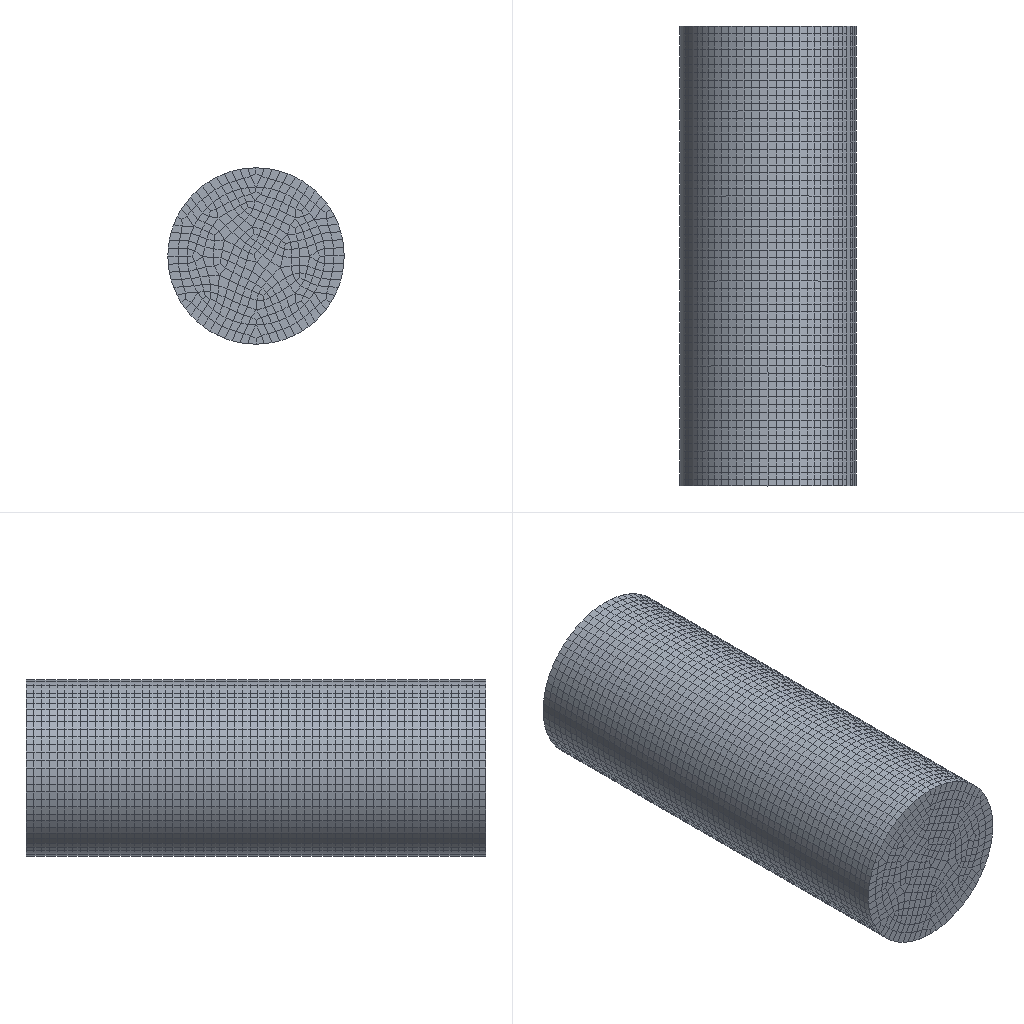Simulation study | ansys workbench
Set-up summary:
category,name,step,type,value,unit,region
solver,ansys_workbench
units,SI m-kg-s (Pa),,stated,"/units,MKS"
analysis,deck-1/LS1,,steady-state thermal
load_step,deck-1/LS1,deck-1/LS1,steady-state thermal,nsubst=1; time=1
analysis,deck-2/LS1,,transient thermal
load_step,deck-2/LS1,deck-2/LS1,transient thermal,nsubst=100; time=10
analysis,deck-3/LS1,,transient thermal
load_step,deck-3/LS1,deck-3/LS1,transient thermal,nsubst=100; time=100
mesh,deck-1.dat,,nodes,46128
mesh,deck-1.dat,,elements,12591
element_type,SOLID90,,,8511,,deck-1.dat
element_type,SURF152,,,4080,,deck-1.dat
mesh,deck-2.dat,,nodes,46128
mesh,deck-2.dat,,elements,12591
element_type,SOLID90,,,8511,,deck-2.dat
element_type,SURF152,,,4080,,deck-2.dat
mesh,deck-3.dat,,nodes,46128
mesh,deck-3.dat,,elements,12591
element_type,SOLID90,,,8511,,deck-3.dat
element_type,SURF152,,,4080,,deck-3.dat
material,Structural Steel,,E,2e+11,Pa
material,Structural Steel,,nu,0.3
material,Structural Steel,,density,7850,kg m^-3
material,Structural Steel,,conductivity,60.5,W m^-1 C^-1
material,Structural Steel,,specific_heat,434,J kg^-1 C^-1
material,Structural Steel,,cte,1.2e-05,C^-1
material,Structural Steel,,permeability,10000
material,Structural Steel,,resistivity,1.7e-07,kg m^3 A^-2 s^-3
load,Define Uniform Initial temperature,deck-1/model,body load temp,22,,all
load,"Create ""______""",deck-1/LS1,convection,250,,SURF152 #2
load,Define Uniform Initial temperature,deck-2/model,body load temp,22,,all
load,"Create ""______""",deck-2/LS1,convection,250,,SURF152 #2
load,"Create ""______""",deck-3/LS1,convection,250,,SURF152 #2
bc,,deck-1/LS1,temperature,100 [dofs=TEMP],,node list
bc,,deck-2/LS1,temperature,100 [dofs=TEMP],,node list
named_set,_CM33,,node,10344
named_set,_CM52,,node,10344
Results summary:
result,analyses[0].index,,,1
result,analyses[0].system,,,SYS
result,analyses[0].deck,,,deck-1.dat
result,analyses[0].solve_status,,,completed
result,analyses[0].analysis_type,,,static
result,analyses[0].physics,,,thermal
result,analyses[0].unit_system,,,"MKS: m, kg, N, s, V, A, degC"
result,analyses[0].n_sets,,,1
result,analyses[0].load_steps[0].set,set=1,,1
result,analyses[0].load_steps[0].time_or_freq,set=1,,1
result,analyses[0].load_steps[0].max_temperature,set=1,,100
result,analyses[0].load_steps[0].min_temperature,set=1,,97.697
result,analyses[1].index,,,2
result,analyses[1].system,,,SYS-1
result,analyses[1].deck,,,deck-2.dat
result,analyses[1].solve_status,,,completed
result,analyses[1].analysis_type,,,static
result,analyses[1].physics,,,thermal
result,analyses[1].unit_system,,,"MKS: m, kg, N, s, V, A, degC"
result,analyses[1].n_sets,,,28
result,analyses[1].load_steps[0].set,set=28,,28
result,analyses[1].load_steps[0].time_or_freq,set=28,,10
result,analyses[1].load_steps[0].max_temperature,set=28,,100
result,analyses[1].load_steps[0].min_temperature,set=28,,97.677
result,analyses[2].index,,,3
result,analyses[2].system,,,SYS-2
result,analyses[2].deck,,,deck-3.dat
result,analyses[2].solve_status,,,completed
result,analyses[2].analysis_type,,,static
result,analyses[2].physics,,,thermal
result,analyses[2].unit_system,,,"MKS: m, kg, N, s, V, A, degC"
result,analyses[2].n_sets,,,13
result,analyses[2].load_steps[0].set,set=13,,13
result,analyses[2].load_steps[0].time_or_freq,set=13,,100
result,analyses[2].load_steps[0].max_temperature,set=13,,45.685
result,analyses[2].load_steps[0].min_temperature,set=13,,38.827
result,geometry_export[0][0],,,.step
result,geometry_export[0][1],,,ok
result,geometry_export[0][2],,,1